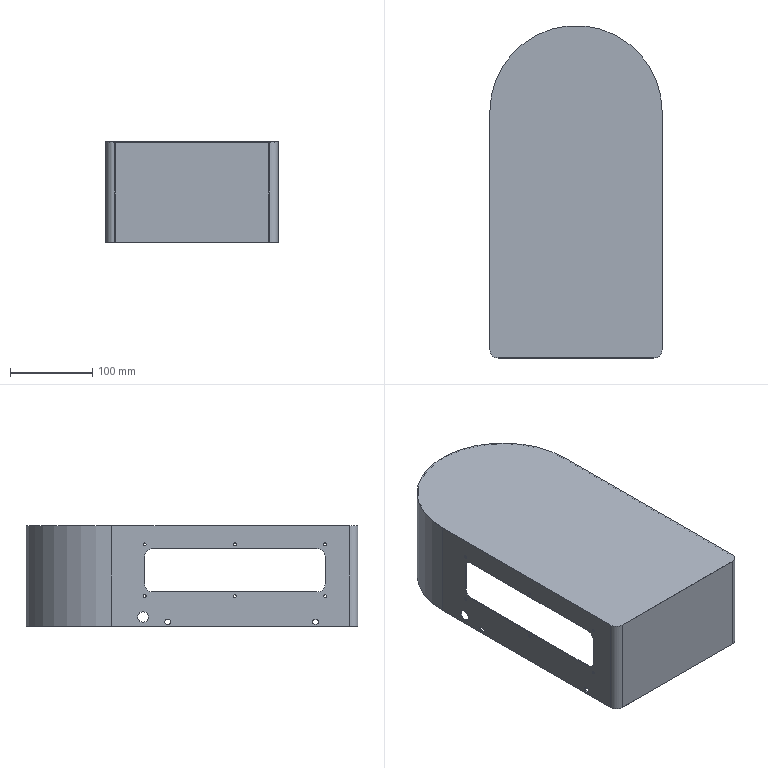Part | SolidWorks | features ICE 5, Fillet 3, Extrusion 1 | 1 solid | 75 faces | box 210 x 405 x 123 mm | volume 233905 mm3 | cylinder 50 | plane 25 | commonest cylinder face diameters 3.5 x24 20 x12 5.5 x8 13 x4 207.6 x1 210 x1